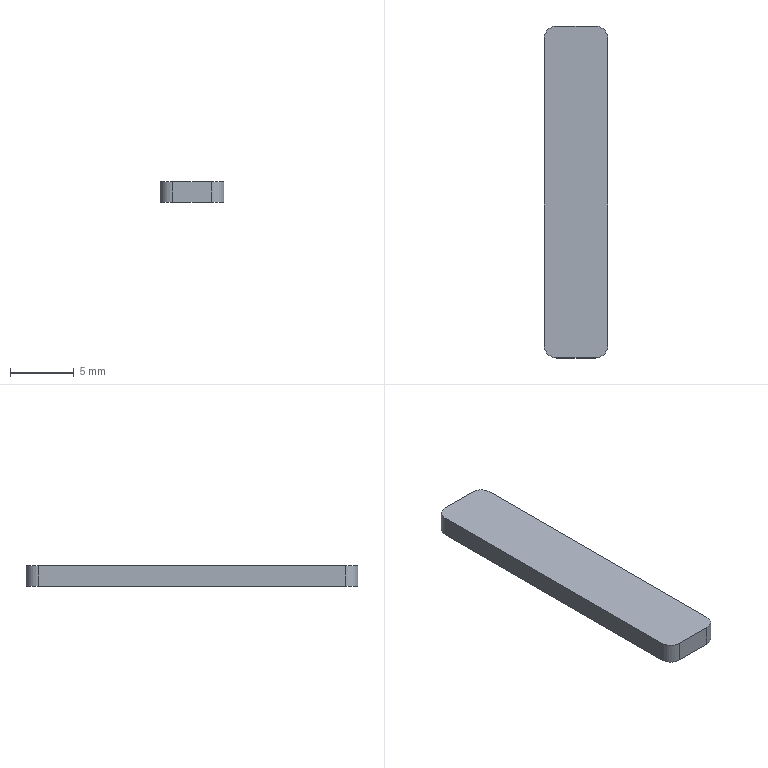Part | SolidWorks | features Fillet 1, FlatPattern 1, SMBaseFlange 1, SheetMetal 1 | 1 solid | 10 faces | box 5 x 26 x 1.6 mm | volume 206.627 mm3 | plane 6 | cylinder 4 | commonest cylinder face diameters 2 x4
STEP:
#1=CARTESIAN_POINT('',(165.,347.7,0.));
#2=VERTEX_POINT('',#1);
#3=CARTESIAN_POINT('',(165.,323.7,0.));
#4=VERTEX_POINT('',#3);
#5=CARTESIAN_POINT('',(165.,348.7,0.));
#6=DIRECTION('',(0.,-1.,0.));
#7=VECTOR('',#6,1000.);
#8=LINE('',#5,#7);
#9=EDGE_CURVE('',#2,#4,#8,.T.);
#10=ORIENTED_EDGE('',*,*,#9,.F.);
#11=CARTESIAN_POINT('',(165.,347.7,-1.6));
#12=VERTEX_POINT('',#11);
#13=CARTESIAN_POINT('',(165.,347.7,-1.6));
#14=DIRECTION('',(0.,0.,-1.));
#15=VECTOR('',#14,1000.);
#16=LINE('',#13,#15);
#17=EDGE_CURVE('',#2,#12,#16,.T.);
#18=ORIENTED_EDGE('',*,*,#17,.T.);
#19=CARTESIAN_POINT('',(165.,323.7,-1.6));
#20=VERTEX_POINT('',#19);
#21=CARTESIAN_POINT('',(165.,348.7,-1.6));
#22=DIRECTION('',(0.,-1.,0.));
#23=VECTOR('',#22,1000.);
#24=LINE('',#21,#23);
#25=EDGE_CURVE('',#12,#20,#24,.T.);
#26=ORIENTED_EDGE('',*,*,#25,.T.);
#27=CARTESIAN_POINT('',(165.,323.7,-1.6));
#28=DIRECTION('',(0.,0.,1.));
#29=VECTOR('',#28,1000.);
#30=LINE('',#27,#29);
#31=EDGE_CURVE('',#20,#4,#30,.T.);
#32=ORIENTED_EDGE('',*,*,#31,.T.);
#33=EDGE_LOOP('',(#10,#18,#26,#32));
#34=FACE_OUTER_BOUND('',#33,.T.);
#35=CARTESIAN_POINT('',(165.,348.7,-1.6));
#36=DIRECTION('',(-1.,0.,0.));
#37=DIRECTION('',(0.,0.,1.));
#38=AXIS2_PLACEMENT_3D('',#35,#36,#37);
#39=PLANE('',#38);
#40=ADVANCED_FACE('',(#34),#39,.T.);
#41=CARTESIAN_POINT('',(169.,348.7,0.));
#42=VERTEX_POINT('',#41);
#43=CARTESIAN_POINT('',(166.,348.7,0.));
#44=VERTEX_POINT('',#43);
#45=CARTESIAN_POINT('',(170.,348.7,0.));
#46=DIRECTION('',(-1.,0.,0.));
#47=VECTOR('',#46,1000.);
#48=LINE('',#45,#47);
#49=EDGE_CURVE('',#42,#44,#48,.T.);
#50=ORIENTED_EDGE('',*,*,#49,.F.);
#51=CARTESIAN_POINT('',(169.,348.7,-1.6));
#52=VERTEX_POINT('',#51);
#53=CARTESIAN_POINT('',(169.,348.7,-1.6));
#54=DIRECTION('',(0.,0.,-1.));
#55=VECTOR('',#54,1000.);
#56=LINE('',#53,#55);
#57=EDGE_CURVE('',#42,#52,#56,.T.);
#58=ORIENTED_EDGE('',*,*,#57,.T.);
#59=CARTESIAN_POINT('',(166.,348.7,-1.6));
#60=VERTEX_POINT('',#59);
#61=CARTESIAN_POINT('',(170.,348.7,-1.6));
#62=DIRECTION('',(-1.,0.,0.));
#63=VECTOR('',#62,1000.);
#64=LINE('',#61,#63);
#65=EDGE_CURVE('',#52,#60,#64,.T.);
#66=ORIENTED_EDGE('',*,*,#65,.T.);
#67=CARTESIAN_POINT('',(166.,348.7,-1.6));
#68=DIRECTION('',(0.,0.,1.));
#69=VECTOR('',#68,1000.);
#70=LINE('',#67,#69);
#71=EDGE_CURVE('',#60,#44,#70,.T.);
#72=ORIENTED_EDGE('',*,*,#71,.T.);
#73=EDGE_LOOP('',(#50,#58,#66,#72));
#74=FACE_OUTER_BOUND('',#73,.T.);
#75=CARTESIAN_POINT('',(170.,348.7,-1.6));
#76=DIRECTION('',(0.,1.,0.));
#77=DIRECTION('',(0.,0.,1.));
#78=AXIS2_PLACEMENT_3D('',#75,#76,#77);
#79=PLANE('',#78);
#80=ADVANCED_FACE('',(#74),#79,.T.);
#81=CARTESIAN_POINT('',(170.,323.7,-1.6));
#82=VERTEX_POINT('',#81);
#83=CARTESIAN_POINT('',(170.,347.7,-1.6));
#84=VERTEX_POINT('',#83);
#85=CARTESIAN_POINT('',(170.,322.7,-1.6));
#86=DIRECTION('',(0.,1.,0.));
#87=VECTOR('',#86,1000.);
#88=LINE('',#85,#87);
#89=EDGE_CURVE('',#82,#84,#88,.T.);
#90=ORIENTED_EDGE('',*,*,#89,.T.);
#91=CARTESIAN_POINT('',(170.,347.7,0.));
#92=VERTEX_POINT('',#91);
#93=CARTESIAN_POINT('',(170.,347.7,-1.6));
#94=DIRECTION('',(0.,0.,1.));
#95=VECTOR('',#94,1000.);
#96=LINE('',#93,#95);
#97=EDGE_CURVE('',#84,#92,#96,.T.);
#98=ORIENTED_EDGE('',*,*,#97,.T.);
#99=CARTESIAN_POINT('',(170.,323.7,0.));
#100=VERTEX_POINT('',#99);
#101=CARTESIAN_POINT('',(170.,322.7,0.));
#102=DIRECTION('',(0.,1.,0.));
#103=VECTOR('',#102,1000.);
#104=LINE('',#101,#103);
#105=EDGE_CURVE('',#100,#92,#104,.T.);
#106=ORIENTED_EDGE('',*,*,#105,.F.);
#107=CARTESIAN_POINT('',(170.,323.7,-1.6));
#108=DIRECTION('',(0.,0.,-1.));
#109=VECTOR('',#108,1000.);
#110=LINE('',#107,#109);
#111=EDGE_CURVE('',#100,#82,#110,.T.);
#112=ORIENTED_EDGE('',*,*,#111,.T.);
#113=EDGE_LOOP('',(#90,#98,#106,#112));
#114=FACE_OUTER_BOUND('',#113,.T.);
#115=CARTESIAN_POINT('',(170.,322.7,-1.6));
#116=DIRECTION('',(1.,0.,0.));
#117=DIRECTION('',(0.,0.,-1.));
#118=AXIS2_PLACEMENT_3D('',#115,#116,#117);
#119=PLANE('',#118);
#120=ADVANCED_FACE('',(#114),#119,.T.);
#121=CARTESIAN_POINT('',(166.,322.7,0.));
#122=VERTEX_POINT('',#121);
#123=CARTESIAN_POINT('',(169.,322.7,0.));
#124=VERTEX_POINT('',#123);
#125=CARTESIAN_POINT('',(165.,322.7,0.));
#126=DIRECTION('',(1.,0.,0.));
#127=VECTOR('',#126,1000.);
#128=LINE('',#125,#127);
#129=EDGE_CURVE('',#122,#124,#128,.T.);
#130=ORIENTED_EDGE('',*,*,#129,.F.);
#131=CARTESIAN_POINT('',(166.,322.7,-1.6));
#132=VERTEX_POINT('',#131);
#133=CARTESIAN_POINT('',(166.,322.7,-1.6));
#134=DIRECTION('',(0.,0.,-1.));
#135=VECTOR('',#134,1000.);
#136=LINE('',#133,#135);
#137=EDGE_CURVE('',#122,#132,#136,.T.);
#138=ORIENTED_EDGE('',*,*,#137,.T.);
#139=CARTESIAN_POINT('',(169.,322.7,-1.6));
#140=VERTEX_POINT('',#139);
#141=CARTESIAN_POINT('',(165.,322.7,-1.6));
#142=DIRECTION('',(1.,0.,0.));
#143=VECTOR('',#142,1000.);
#144=LINE('',#141,#143);
#145=EDGE_CURVE('',#132,#140,#144,.T.);
#146=ORIENTED_EDGE('',*,*,#145,.T.);
#147=CARTESIAN_POINT('',(169.,322.7,-1.6));
#148=DIRECTION('',(0.,0.,1.));
#149=VECTOR('',#148,1000.);
#150=LINE('',#147,#149);
#151=EDGE_CURVE('',#140,#124,#150,.T.);
#152=ORIENTED_EDGE('',*,*,#151,.T.);
#153=EDGE_LOOP('',(#130,#138,#146,#152));
#154=FACE_OUTER_BOUND('',#153,.T.);
#155=CARTESIAN_POINT('',(165.,322.7,-1.6));
#156=DIRECTION('',(0.,-1.,0.));
#157=DIRECTION('',(0.,0.,-1.));
#158=AXIS2_PLACEMENT_3D('',#155,#156,#157);
#159=PLANE('',#158);
#160=ADVANCED_FACE('',(#154),#159,.T.);
#161=ORIENTED_EDGE('',*,*,#65,.F.);
#162=CARTESIAN_POINT('',(169.,347.7,-1.6));
#163=DIRECTION('',(0.,0.,-1.));
#164=DIRECTION('',(1.,0.,0.));
#165=AXIS2_PLACEMENT_3D('',#162,#163,#164);
#166=CIRCLE('',#165,1.);
#167=EDGE_CURVE('',#52,#84,#166,.T.);
#168=ORIENTED_EDGE('',*,*,#167,.T.);
#169=ORIENTED_EDGE('',*,*,#89,.F.);
#170=CARTESIAN_POINT('',(169.,323.7,-1.6));
#171=DIRECTION('',(0.,0.,-1.));
#172=DIRECTION('',(1.,0.,0.));
#173=AXIS2_PLACEMENT_3D('',#170,#171,#172);
#174=CIRCLE('',#173,1.);
#175=EDGE_CURVE('',#82,#140,#174,.T.);
#176=ORIENTED_EDGE('',*,*,#175,.T.);
#177=ORIENTED_EDGE('',*,*,#145,.F.);
#178=CARTESIAN_POINT('',(166.,323.7,-1.6));
#179=DIRECTION('',(0.,0.,-1.));
#180=DIRECTION('',(1.,0.,0.));
#181=AXIS2_PLACEMENT_3D('',#178,#179,#180);
#182=CIRCLE('',#181,1.);
#183=EDGE_CURVE('',#132,#20,#182,.T.);
#184=ORIENTED_EDGE('',*,*,#183,.T.);
#185=ORIENTED_EDGE('',*,*,#25,.F.);
#186=CARTESIAN_POINT('',(166.,347.7,-1.6));
#187=DIRECTION('',(0.,0.,-1.));
#188=DIRECTION('',(1.,0.,0.));
#189=AXIS2_PLACEMENT_3D('',#186,#187,#188);
#190=CIRCLE('',#189,1.);
#191=EDGE_CURVE('',#12,#60,#190,.T.);
#192=ORIENTED_EDGE('',*,*,#191,.T.);
#193=EDGE_LOOP('',(#161,#168,#169,#176,#177,#184,#185,#192));
#194=FACE_OUTER_BOUND('',#193,.T.);
#195=CARTESIAN_POINT('',(0.,0.,-1.6));
#196=DIRECTION('',(0.,0.,1.));
#197=DIRECTION('',(1.,0.,0.));
#198=AXIS2_PLACEMENT_3D('',#195,#196,#197);
#199=PLANE('',#198);
#200=ADVANCED_FACE('',(#194),#199,.F.);
#201=ORIENTED_EDGE('',*,*,#105,.T.);
#202=CARTESIAN_POINT('',(169.,347.7,0.));
#203=DIRECTION('',(0.,0.,1.));
#204=DIRECTION('',(1.,0.,0.));
#205=AXIS2_PLACEMENT_3D('',#202,#203,#204);
#206=CIRCLE('',#205,1.);
#207=EDGE_CURVE('',#92,#42,#206,.T.);
#208=ORIENTED_EDGE('',*,*,#207,.T.);
#209=ORIENTED_EDGE('',*,*,#49,.T.);
#210=CARTESIAN_POINT('',(166.,347.7,0.));
#211=DIRECTION('',(0.,0.,1.));
#212=DIRECTION('',(1.,0.,0.));
#213=AXIS2_PLACEMENT_3D('',#210,#211,#212);
#214=CIRCLE('',#213,1.);
#215=EDGE_CURVE('',#44,#2,#214,.T.);
#216=ORIENTED_EDGE('',*,*,#215,.T.);
#217=ORIENTED_EDGE('',*,*,#9,.T.);
#218=CARTESIAN_POINT('',(166.,323.7,0.));
#219=DIRECTION('',(0.,0.,1.));
#220=DIRECTION('',(1.,0.,0.));
#221=AXIS2_PLACEMENT_3D('',#218,#219,#220);
#222=CIRCLE('',#221,1.);
#223=EDGE_CURVE('',#4,#122,#222,.T.);
#224=ORIENTED_EDGE('',*,*,#223,.T.);
#225=ORIENTED_EDGE('',*,*,#129,.T.);
#226=CARTESIAN_POINT('',(169.,323.7,0.));
#227=DIRECTION('',(0.,0.,1.));
#228=DIRECTION('',(1.,0.,0.));
#229=AXIS2_PLACEMENT_3D('',#226,#227,#228);
#230=CIRCLE('',#229,1.);
#231=EDGE_CURVE('',#124,#100,#230,.T.);
#232=ORIENTED_EDGE('',*,*,#231,.T.);
#233=EDGE_LOOP('',(#201,#208,#209,#216,#217,#224,#225,#232));
#234=FACE_OUTER_BOUND('',#233,.T.);
#235=CARTESIAN_POINT('',(0.,0.,0.));
#236=DIRECTION('',(0.,0.,1.));
#237=DIRECTION('',(1.,0.,0.));
#238=AXIS2_PLACEMENT_3D('',#235,#236,#237);
#239=PLANE('',#238);
#240=ADVANCED_FACE('',(#234),#239,.T.);
#241=ORIENTED_EDGE('',*,*,#167,.F.);
#242=ORIENTED_EDGE('',*,*,#57,.F.);
#243=ORIENTED_EDGE('',*,*,#207,.F.);
#244=ORIENTED_EDGE('',*,*,#97,.F.);
#245=EDGE_LOOP('',(#241,#242,#243,#244));
#246=FACE_OUTER_BOUND('',#245,.T.);
#247=CARTESIAN_POINT('',(169.,347.7,-1.6));
#248=DIRECTION('',(0.,0.,1.));
#249=DIRECTION('',(1.,0.,0.));
#250=AXIS2_PLACEMENT_3D('',#247,#248,#249);
#251=CYLINDRICAL_SURFACE('',#250,1.);
#252=ADVANCED_FACE('',(#246),#251,.T.);
#253=ORIENTED_EDGE('',*,*,#191,.F.);
#254=ORIENTED_EDGE('',*,*,#17,.F.);
#255=ORIENTED_EDGE('',*,*,#215,.F.);
#256=ORIENTED_EDGE('',*,*,#71,.F.);
#257=EDGE_LOOP('',(#253,#254,#255,#256));
#258=FACE_OUTER_BOUND('',#257,.T.);
#259=CARTESIAN_POINT('',(166.,347.7,-1.6));
#260=DIRECTION('',(0.,0.,1.));
#261=DIRECTION('',(1.,0.,0.));
#262=AXIS2_PLACEMENT_3D('',#259,#260,#261);
#263=CYLINDRICAL_SURFACE('',#262,1.);
#264=ADVANCED_FACE('',(#258),#263,.T.);
#265=ORIENTED_EDGE('',*,*,#183,.F.);
#266=ORIENTED_EDGE('',*,*,#137,.F.);
#267=ORIENTED_EDGE('',*,*,#223,.F.);
#268=ORIENTED_EDGE('',*,*,#31,.F.);
#269=EDGE_LOOP('',(#265,#266,#267,#268));
#270=FACE_OUTER_BOUND('',#269,.T.);
#271=CARTESIAN_POINT('',(166.,323.7,-1.6));
#272=DIRECTION('',(0.,0.,1.));
#273=DIRECTION('',(1.,0.,0.));
#274=AXIS2_PLACEMENT_3D('',#271,#272,#273);
#275=CYLINDRICAL_SURFACE('',#274,1.);
#276=ADVANCED_FACE('',(#270),#275,.T.);
#277=ORIENTED_EDGE('',*,*,#175,.F.);
#278=ORIENTED_EDGE('',*,*,#111,.F.);
#279=ORIENTED_EDGE('',*,*,#231,.F.);
#280=ORIENTED_EDGE('',*,*,#151,.F.);
#281=EDGE_LOOP('',(#277,#278,#279,#280));
#282=FACE_OUTER_BOUND('',#281,.T.);
#283=CARTESIAN_POINT('',(169.,323.7,-1.6));
#284=DIRECTION('',(0.,0.,1.));
#285=DIRECTION('',(1.,0.,0.));
#286=AXIS2_PLACEMENT_3D('',#283,#284,#285);
#287=CYLINDRICAL_SURFACE('',#286,1.);
#288=ADVANCED_FACE('',(#282),#287,.T.);
#289=CLOSED_SHELL('',(#40,#80,#120,#160,#200,#240,#252,#264,#276,#288));
#290=MANIFOLD_SOLID_BREP('',#289);
#291=CARTESIAN_POINT('',(0.,0.,0.));
#292=DIRECTION('',(0.,0.,1.));
#293=DIRECTION('',(1.,0.,0.));
#294=AXIS2_PLACEMENT_3D('',#291,#292,#293);
#295=(LENGTH_UNIT()NAMED_UNIT(*)SI_UNIT(.MILLI.,.METRE.));
#296=UNCERTAINTY_MEASURE_WITH_UNIT(LENGTH_MEASURE(0.00001),#295,'','');
#297=(NAMED_UNIT(*)PLANE_ANGLE_UNIT()SI_UNIT($,.RADIAN.));
#298=(NAMED_UNIT(*)SI_UNIT($,.STERADIAN.)SOLID_ANGLE_UNIT());
#299=(GEOMETRIC_REPRESENTATION_CONTEXT(3)GLOBAL_UNCERTAINTY_ASSIGNED_CONTEXT((#296))GLOBAL_UNIT_ASSIGNED_CONTEXT((#295,#297,#298))REPRESENTATION_CONTEXT('',''));
#300=ADVANCED_BREP_SHAPE_REPRESENTATION('',(#290,#294),#299);